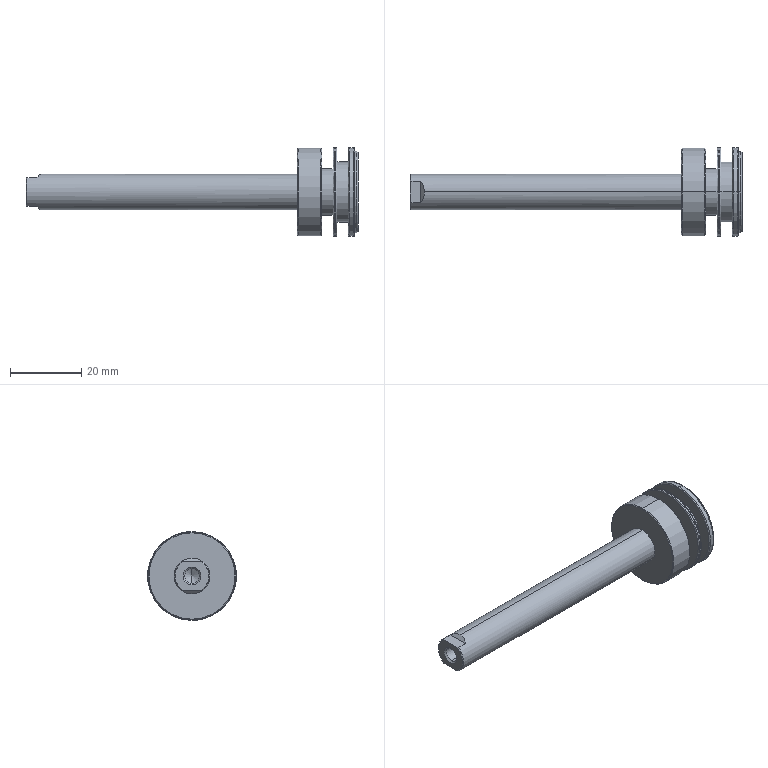Part | STEP file | SDA25x60S-02-cc | 1 solid | 48 faces | box 93 x 24.9 x 24.9 mm | volume 11912 mm3 | cylinder 16 | cone 12 | plane 12 | spline 8 | commonest cylinder face diameters 24.9 x4 4.134 x2 10 x2 13 x2 16.9 x2 22.9 x2